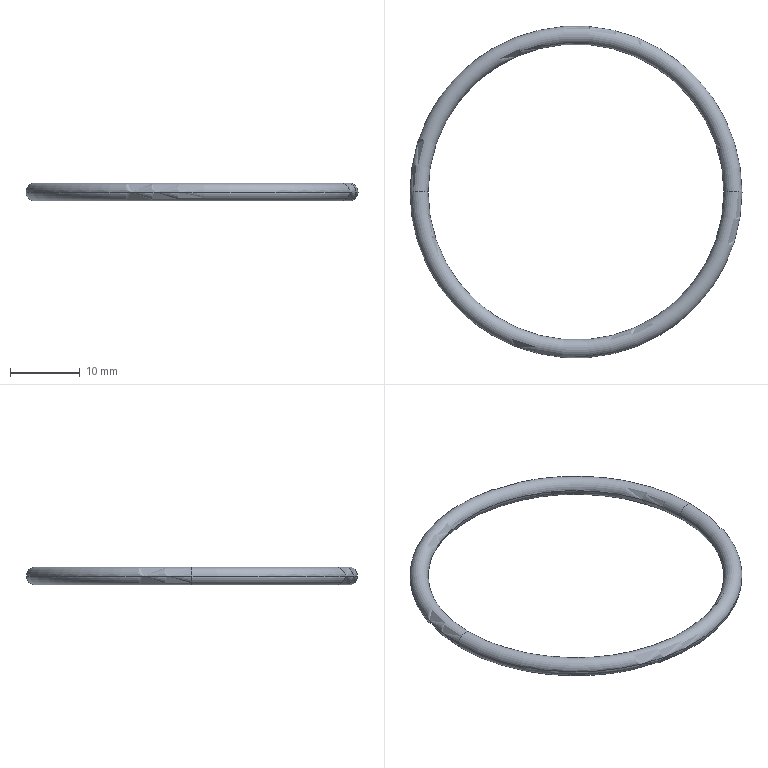Part | STEP file | Inner dia 42.5 wire dia 2.65 O-ring | 1 solid | 4 faces | box 47.7 x 47.7 x 2.6 mm | volume 752.251 mm3 | torus 4
STEP:
#1=CARTESIAN_POINT('',(0.,0.,0.));
#2=DIRECTION('',(0.,0.,1.));
#3=DIRECTION('',(1.,0.,0.));
#4=AXIS2_PLACEMENT_3D('',#1,#2,#3);
#5=CARTESIAN_POINT('',(-23.85,0.,0.));
#6=VERTEX_POINT('',#5);
#7=CARTESIAN_POINT('',(-21.25,0.,0.));
#8=VERTEX_POINT('',#7);
#9=CARTESIAN_POINT('',(-22.55,0.,0.));
#10=DIRECTION('',(0.,1.,0.));
#11=DIRECTION('',(-1.,0.,0.));
#12=AXIS2_PLACEMENT_3D('',#9,#10,#11);
#13=CIRCLE('',#12,1.3);
#14=CARTESIAN_POINT('',(0.,0.,0.));
#15=DIRECTION('',(0.,0.,1.));
#16=DIRECTION('',(1.,0.,0.));
#17=AXIS2_PLACEMENT_3D('',#14,#15,#16);
#18=TOROIDAL_SURFACE('',#17,22.55,1.3);
#19=CARTESIAN_POINT('',(3.142,0.));
#20=DIRECTION('',(0.,1.));
#21=VECTOR('',#20,1.);
#22=LINE('',#19,#21);
#23=(GEOMETRIC_REPRESENTATION_CONTEXT(2)PARAMETRIC_REPRESENTATION_CONTEXT()REPRESENTATION_CONTEXT('',''));
#24=DEFINITIONAL_REPRESENTATION('',(#22),#23);
#25=PCURVE('',#18,#24);
#26=CARTESIAN_POINT('',(0.,0.,0.));
#27=DIRECTION('',(0.,0.,1.));
#28=DIRECTION('',(1.,0.,0.));
#29=AXIS2_PLACEMENT_3D('',#26,#27,#28);
#30=TOROIDAL_SURFACE('',#29,22.55,1.3);
#31=CARTESIAN_POINT('',(3.142,0.));
#32=DIRECTION('',(0.,1.));
#33=VECTOR('',#32,1.);
#34=LINE('',#31,#33);
#35=(GEOMETRIC_REPRESENTATION_CONTEXT(2)PARAMETRIC_REPRESENTATION_CONTEXT()REPRESENTATION_CONTEXT('',''));
#36=DEFINITIONAL_REPRESENTATION('',(#34),#35);
#37=PCURVE('',#30,#36);
#38=SURFACE_CURVE('',#13,(#25,#37),.PCURVE_S1.);
#39=EDGE_CURVE('',#6,#8,#38,.T.);
#40=ORIENTED_EDGE('',*,*,#39,.F.);
#41=CARTESIAN_POINT('',(23.85,0.,0.));
#42=VERTEX_POINT('',#41);
#43=CARTESIAN_POINT('',(0.,0.,0.));
#44=DIRECTION('',(0.,0.,1.));
#45=DIRECTION('',(1.,0.,0.));
#46=AXIS2_PLACEMENT_3D('',#43,#44,#45);
#47=CIRCLE('',#46,23.85);
#48=CARTESIAN_POINT('',(0.,0.));
#49=DIRECTION('',(1.,0.));
#50=VECTOR('',#49,1.);
#51=LINE('',#48,#50);
#52=(GEOMETRIC_REPRESENTATION_CONTEXT(2)PARAMETRIC_REPRESENTATION_CONTEXT()REPRESENTATION_CONTEXT('',''));
#53=DEFINITIONAL_REPRESENTATION('',(#51),#52);
#54=PCURVE('',#18,#53);
#55=CARTESIAN_POINT('',(0.,0.,0.));
#56=DIRECTION('',(0.,0.,1.));
#57=DIRECTION('',(1.,0.,0.));
#58=AXIS2_PLACEMENT_3D('',#55,#56,#57);
#59=TOROIDAL_SURFACE('',#58,22.55,1.3);
#60=CARTESIAN_POINT('',(0.,6.283));
#61=DIRECTION('',(1.,0.));
#62=VECTOR('',#61,1.);
#63=LINE('',#60,#62);
#64=(GEOMETRIC_REPRESENTATION_CONTEXT(2)PARAMETRIC_REPRESENTATION_CONTEXT()REPRESENTATION_CONTEXT('',''));
#65=DEFINITIONAL_REPRESENTATION('',(#63),#64);
#66=PCURVE('',#59,#65);
#67=SURFACE_CURVE('',#47,(#54,#66),.PCURVE_S1.);
#68=EDGE_CURVE('',#6,#42,#67,.T.);
#69=ORIENTED_EDGE('',*,*,#68,.T.);
#70=CARTESIAN_POINT('',(21.25,0.,0.));
#71=VERTEX_POINT('',#70);
#72=CARTESIAN_POINT('',(22.55,0.,0.));
#73=DIRECTION('',(0.,-1.,0.));
#74=DIRECTION('',(0.,0.,-1.));
#75=AXIS2_PLACEMENT_3D('',#72,#73,#74);
#76=CIRCLE('',#75,1.3);
#77=CARTESIAN_POINT('',(6.283,-1.571));
#78=DIRECTION('',(0.,1.));
#79=VECTOR('',#78,1.);
#80=LINE('',#77,#79);
#81=(GEOMETRIC_REPRESENTATION_CONTEXT(2)PARAMETRIC_REPRESENTATION_CONTEXT()REPRESENTATION_CONTEXT('',''));
#82=DEFINITIONAL_REPRESENTATION('',(#80),#81);
#83=PCURVE('',#18,#82);
#84=CARTESIAN_POINT('',(0.,-1.571));
#85=DIRECTION('',(0.,1.));
#86=VECTOR('',#85,1.);
#87=LINE('',#84,#86);
#88=(GEOMETRIC_REPRESENTATION_CONTEXT(2)PARAMETRIC_REPRESENTATION_CONTEXT()REPRESENTATION_CONTEXT('',''));
#89=DEFINITIONAL_REPRESENTATION('',(#87),#88);
#90=PCURVE('',#30,#89);
#91=SURFACE_CURVE('',#76,(#83,#90),.PCURVE_S1.);
#92=EDGE_CURVE('',#42,#71,#91,.T.);
#93=ORIENTED_EDGE('',*,*,#92,.T.);
#94=CARTESIAN_POINT('',(0.,0.,0.));
#95=DIRECTION('',(0.,0.,1.));
#96=DIRECTION('',(1.,0.,0.));
#97=AXIS2_PLACEMENT_3D('',#94,#95,#96);
#98=CIRCLE('',#97,21.25);
#99=CARTESIAN_POINT('',(0.,3.142));
#100=DIRECTION('',(1.,0.));
#101=VECTOR('',#100,1.);
#102=LINE('',#99,#101);
#103=(GEOMETRIC_REPRESENTATION_CONTEXT(2)PARAMETRIC_REPRESENTATION_CONTEXT()REPRESENTATION_CONTEXT('',''));
#104=DEFINITIONAL_REPRESENTATION('',(#102),#103);
#105=PCURVE('',#18,#104);
#106=CARTESIAN_POINT('',(0.,3.142));
#107=DIRECTION('',(1.,0.));
#108=VECTOR('',#107,1.);
#109=LINE('',#106,#108);
#110=(GEOMETRIC_REPRESENTATION_CONTEXT(2)PARAMETRIC_REPRESENTATION_CONTEXT()REPRESENTATION_CONTEXT('',''));
#111=DEFINITIONAL_REPRESENTATION('',(#109),#110);
#112=PCURVE('',#59,#111);
#113=SURFACE_CURVE('',#98,(#105,#112),.PCURVE_S1.);
#114=EDGE_CURVE('',#8,#71,#113,.T.);
#115=ORIENTED_EDGE('',*,*,#114,.F.);
#116=EDGE_LOOP('',(#40,#69,#93,#115));
#117=FACE_BOUND('',#116,.T.);
#118=ADVANCED_FACE('',(#117),#18,.T.);
#119=ORIENTED_EDGE('',*,*,#92,.F.);
#120=CARTESIAN_POINT('',(0.,0.,0.));
#121=DIRECTION('',(0.,0.,1.));
#122=DIRECTION('',(1.,0.,0.));
#123=AXIS2_PLACEMENT_3D('',#120,#121,#122);
#124=CIRCLE('',#123,23.85);
#125=CARTESIAN_POINT('',(0.,0.));
#126=DIRECTION('',(1.,0.));
#127=VECTOR('',#126,1.);
#128=LINE('',#125,#127);
#129=(GEOMETRIC_REPRESENTATION_CONTEXT(2)PARAMETRIC_REPRESENTATION_CONTEXT()REPRESENTATION_CONTEXT('',''));
#130=DEFINITIONAL_REPRESENTATION('',(#128),#129);
#131=PCURVE('',#30,#130);
#132=CARTESIAN_POINT('',(0.,0.,0.));
#133=DIRECTION('',(0.,0.,1.));
#134=DIRECTION('',(1.,0.,0.));
#135=AXIS2_PLACEMENT_3D('',#132,#133,#134);
#136=TOROIDAL_SURFACE('',#135,22.55,1.3);
#137=CARTESIAN_POINT('',(0.,6.283));
#138=DIRECTION('',(1.,0.));
#139=VECTOR('',#138,1.);
#140=LINE('',#137,#139);
#141=(GEOMETRIC_REPRESENTATION_CONTEXT(2)PARAMETRIC_REPRESENTATION_CONTEXT()REPRESENTATION_CONTEXT('',''));
#142=DEFINITIONAL_REPRESENTATION('',(#140),#141);
#143=PCURVE('',#136,#142);
#144=SURFACE_CURVE('',#124,(#131,#143),.PCURVE_S1.);
#145=EDGE_CURVE('',#42,#6,#144,.T.);
#146=ORIENTED_EDGE('',*,*,#145,.T.);
#147=ORIENTED_EDGE('',*,*,#39,.T.);
#148=CARTESIAN_POINT('',(0.,0.,0.));
#149=DIRECTION('',(0.,0.,1.));
#150=DIRECTION('',(1.,0.,0.));
#151=AXIS2_PLACEMENT_3D('',#148,#149,#150);
#152=CIRCLE('',#151,21.25);
#153=CARTESIAN_POINT('',(0.,3.142));
#154=DIRECTION('',(1.,0.));
#155=VECTOR('',#154,1.);
#156=LINE('',#153,#155);
#157=(GEOMETRIC_REPRESENTATION_CONTEXT(2)PARAMETRIC_REPRESENTATION_CONTEXT()REPRESENTATION_CONTEXT('',''));
#158=DEFINITIONAL_REPRESENTATION('',(#156),#157);
#159=PCURVE('',#30,#158);
#160=CARTESIAN_POINT('',(0.,3.142));
#161=DIRECTION('',(1.,0.));
#162=VECTOR('',#161,1.);
#163=LINE('',#160,#162);
#164=(GEOMETRIC_REPRESENTATION_CONTEXT(2)PARAMETRIC_REPRESENTATION_CONTEXT()REPRESENTATION_CONTEXT('',''));
#165=DEFINITIONAL_REPRESENTATION('',(#163),#164);
#166=PCURVE('',#136,#165);
#167=SURFACE_CURVE('',#152,(#159,#166),.PCURVE_S1.);
#168=EDGE_CURVE('',#71,#8,#167,.T.);
#169=ORIENTED_EDGE('',*,*,#168,.F.);
#170=EDGE_LOOP('',(#119,#146,#147,#169));
#171=FACE_BOUND('',#170,.T.);
#172=ADVANCED_FACE('',(#171),#30,.T.);
#173=ORIENTED_EDGE('',*,*,#145,.F.);
#174=CARTESIAN_POINT('',(22.55,0.,0.));
#175=DIRECTION('',(0.,-1.,0.));
#176=DIRECTION('',(0.,0.,-1.));
#177=AXIS2_PLACEMENT_3D('',#174,#175,#176);
#178=CIRCLE('',#177,1.3);
#179=CARTESIAN_POINT('',(0.,-1.571));
#180=DIRECTION('',(0.,1.));
#181=VECTOR('',#180,1.);
#182=LINE('',#179,#181);
#183=(GEOMETRIC_REPRESENTATION_CONTEXT(2)PARAMETRIC_REPRESENTATION_CONTEXT()REPRESENTATION_CONTEXT('',''));
#184=DEFINITIONAL_REPRESENTATION('',(#182),#183);
#185=PCURVE('',#136,#184);
#186=CARTESIAN_POINT('',(6.283,-1.571));
#187=DIRECTION('',(0.,1.));
#188=VECTOR('',#187,1.);
#189=LINE('',#186,#188);
#190=(GEOMETRIC_REPRESENTATION_CONTEXT(2)PARAMETRIC_REPRESENTATION_CONTEXT()REPRESENTATION_CONTEXT('',''));
#191=DEFINITIONAL_REPRESENTATION('',(#189),#190);
#192=PCURVE('',#59,#191);
#193=SURFACE_CURVE('',#178,(#185,#192),.PCURVE_S1.);
#194=EDGE_CURVE('',#71,#42,#193,.T.);
#195=ORIENTED_EDGE('',*,*,#194,.F.);
#196=ORIENTED_EDGE('',*,*,#168,.T.);
#197=CARTESIAN_POINT('',(-22.55,0.,0.));
#198=DIRECTION('',(0.,1.,0.));
#199=DIRECTION('',(-1.,0.,0.));
#200=AXIS2_PLACEMENT_3D('',#197,#198,#199);
#201=CIRCLE('',#200,1.3);
#202=CARTESIAN_POINT('',(3.142,0.));
#203=DIRECTION('',(0.,1.));
#204=VECTOR('',#203,1.);
#205=LINE('',#202,#204);
#206=(GEOMETRIC_REPRESENTATION_CONTEXT(2)PARAMETRIC_REPRESENTATION_CONTEXT()REPRESENTATION_CONTEXT('',''));
#207=DEFINITIONAL_REPRESENTATION('',(#205),#206);
#208=PCURVE('',#136,#207);
#209=CARTESIAN_POINT('',(3.142,0.));
#210=DIRECTION('',(0.,1.));
#211=VECTOR('',#210,1.);
#212=LINE('',#209,#211);
#213=(GEOMETRIC_REPRESENTATION_CONTEXT(2)PARAMETRIC_REPRESENTATION_CONTEXT()REPRESENTATION_CONTEXT('',''));
#214=DEFINITIONAL_REPRESENTATION('',(#212),#213);
#215=PCURVE('',#59,#214);
#216=SURFACE_CURVE('',#201,(#208,#215),.PCURVE_S1.);
#217=EDGE_CURVE('',#8,#6,#216,.T.);
#218=ORIENTED_EDGE('',*,*,#217,.T.);
#219=EDGE_LOOP('',(#173,#195,#196,#218));
#220=FACE_BOUND('',#219,.T.);
#221=ADVANCED_FACE('',(#220),#136,.T.);
#222=ORIENTED_EDGE('',*,*,#68,.F.);
#223=ORIENTED_EDGE('',*,*,#217,.F.);
#224=ORIENTED_EDGE('',*,*,#114,.T.);
#225=ORIENTED_EDGE('',*,*,#194,.T.);
#226=EDGE_LOOP('',(#222,#223,#224,#225));
#227=FACE_BOUND('',#226,.T.);
#228=ADVANCED_FACE('',(#227),#59,.T.);
#229=CLOSED_SHELL('',(#118,#172,#221,#228));
#230=MANIFOLD_SOLID_BREP('',#229);
#231=(LENGTH_UNIT()NAMED_UNIT(*)SI_UNIT(.MILLI.,.METRE.));
#232=UNCERTAINTY_MEASURE_WITH_UNIT(LENGTH_MEASURE(0.0000001),#231,'','');
#233=(NAMED_UNIT(*)PLANE_ANGLE_UNIT()SI_UNIT($,.RADIAN.));
#234=(NAMED_UNIT(*)SI_UNIT($,.STERADIAN.)SOLID_ANGLE_UNIT());
#235=(GEOMETRIC_REPRESENTATION_CONTEXT(3)GLOBAL_UNCERTAINTY_ASSIGNED_CONTEXT((#232))GLOBAL_UNIT_ASSIGNED_CONTEXT((#231,#233,#234))REPRESENTATION_CONTEXT('',''));
#236=ADVANCED_BREP_SHAPE_REPRESENTATION('',(#4,#230),#235);